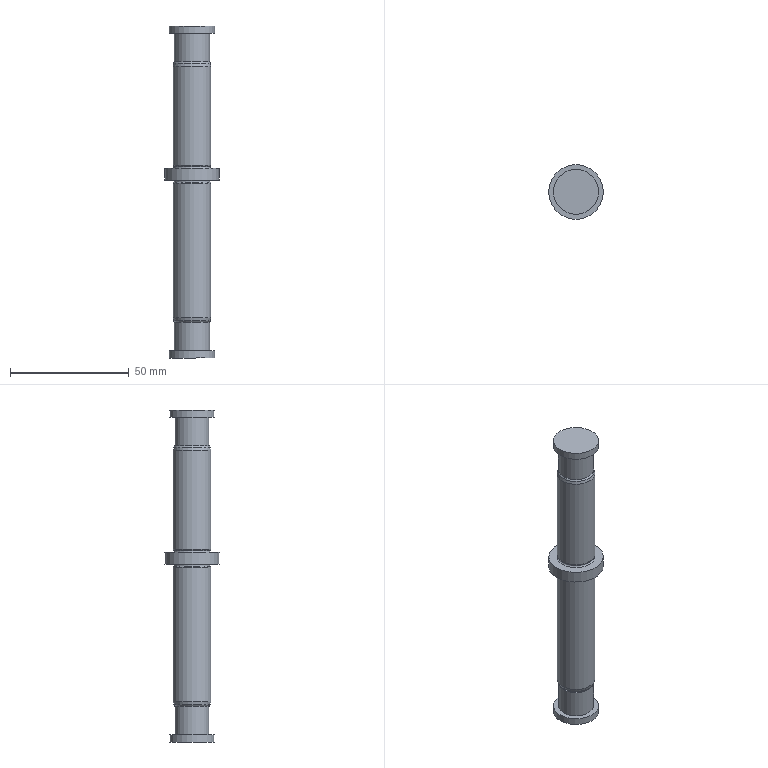Part | STEP file | 200 mesh_id1798 | 1 solid | 23 faces | box 23 x 23 x 140 mm | volume 28914 mm3 | plane 8 | cylinder 7 | torus 6 | cone 2 | commonest cylinder face diameters 14.8 x2 16 x2 19 x2 23 x1
STEP:
#1=CARTESIAN_POINT('',(-17045.208,-4095.269,118.667));
#2=VERTEX_POINT('',#1);
#3=CARTESIAN_POINT('',(-17052.884,-4095.269,118.667));
#4=DIRECTION('',(0.,0.,-1.));
#5=DIRECTION('',(1.,0.,0.));
#6=AXIS2_PLACEMENT_3D('',#3,#4,#5);
#7=CIRCLE('',#6,7.676);
#8=EDGE_CURVE('',#2,#2,#7,.T.);
#9=ORIENTED_EDGE('',*,*,#8,.T.);
#10=EDGE_LOOP('',(#9));
#11=FACE_BOUND('',#10,.T.);
#12=CARTESIAN_POINT('',(-17060.884,-4095.269,117.458));
#13=VERTEX_POINT('',#12);
#14=CARTESIAN_POINT('',(-17052.884,-4095.269,117.458));
#15=DIRECTION('',(0.,0.,-1.));
#16=DIRECTION('',(-1.,0.,0.));
#17=AXIS2_PLACEMENT_3D('',#14,#15,#16);
#18=CIRCLE('',#17,8.);
#19=EDGE_CURVE('',#13,#13,#18,.T.);
#20=ORIENTED_EDGE('',*,*,#19,.F.);
#21=EDGE_LOOP('',(#20));
#22=FACE_BOUND('',#21,.T.);
#23=CARTESIAN_POINT('',(-17052.884,-4095.269,117.458));
#24=DIRECTION('',(0.,0.,-1.));
#25=DIRECTION('',(-1.,0.,0.));
#26=AXIS2_PLACEMENT_3D('',#23,#24,#25);
#27=CONICAL_SURFACE('',#26,8.,15.);
#28=ADVANCED_FACE('',(#11,#22),#27,.T.);
#29=ORIENTED_EDGE('',*,*,#19,.T.);
#30=EDGE_LOOP('',(#29));
#31=FACE_BOUND('',#30,.T.);
#32=CARTESIAN_POINT('',(-17060.884,-4095.269,75.824));
#33=VERTEX_POINT('',#32);
#34=CARTESIAN_POINT('',(-17052.884,-4095.269,75.824));
#35=DIRECTION('',(0.,0.,-1.));
#36=DIRECTION('',(-1.,0.,0.));
#37=AXIS2_PLACEMENT_3D('',#34,#35,#36);
#38=CIRCLE('',#37,8.);
#39=EDGE_CURVE('',#33,#33,#38,.T.);
#40=ORIENTED_EDGE('',*,*,#39,.F.);
#41=EDGE_LOOP('',(#40));
#42=FACE_BOUND('',#41,.T.);
#43=CARTESIAN_POINT('',(-17052.884,-4095.269,74.458));
#44=DIRECTION('',(0.,0.,-1.));
#45=DIRECTION('',(-1.,0.,0.));
#46=AXIS2_PLACEMENT_3D('',#43,#44,#45);
#47=CYLINDRICAL_SURFACE('',#46,8.);
#48=ADVANCED_FACE('',(#31,#42),#47,.T.);
#49=ORIENTED_EDGE('',*,*,#39,.T.);
#50=EDGE_LOOP('',(#49));
#51=FACE_BOUND('',#50,.T.);
#52=CARTESIAN_POINT('',(-17060.634,-4095.269,75.391));
#53=VERTEX_POINT('',#52);
#54=CARTESIAN_POINT('',(-17052.884,-4095.269,75.391));
#55=DIRECTION('',(0.,0.,-1.));
#56=DIRECTION('',(-1.,0.,0.));
#57=AXIS2_PLACEMENT_3D('',#54,#55,#56);
#58=CIRCLE('',#57,7.75);
#59=EDGE_CURVE('',#53,#53,#58,.T.);
#60=ORIENTED_EDGE('',*,*,#59,.F.);
#61=EDGE_LOOP('',(#60));
#62=FACE_BOUND('',#61,.T.);
#63=CARTESIAN_POINT('',(-17052.884,-4095.269,75.824));
#64=DIRECTION('',(0.,0.,-1.));
#65=DIRECTION('',(-1.,0.,0.));
#66=AXIS2_PLACEMENT_3D('',#63,#64,#65);
#67=TOROIDAL_SURFACE('',#66,7.5,0.5);
#68=ADVANCED_FACE('',(#51,#62),#67,.T.);
#69=ORIENTED_EDGE('',*,*,#59,.T.);
#70=EDGE_LOOP('',(#69));
#71=FACE_BOUND('',#70,.T.);
#72=CARTESIAN_POINT('',(-17060.884,-4095.269,74.458));
#73=VERTEX_POINT('',#72);
#74=CARTESIAN_POINT('',(-17052.884,-4095.269,74.458));
#75=DIRECTION('',(0.,0.,-1.));
#76=DIRECTION('',(-1.,0.,0.));
#77=AXIS2_PLACEMENT_3D('',#74,#75,#76);
#78=CIRCLE('',#77,8.);
#79=EDGE_CURVE('',#73,#73,#78,.T.);
#80=ORIENTED_EDGE('',*,*,#79,.F.);
#81=EDGE_LOOP('',(#80));
#82=FACE_BOUND('',#81,.T.);
#83=CARTESIAN_POINT('',(-17052.884,-4095.269,74.958));
#84=DIRECTION('',(0.,0.,-1.));
#85=DIRECTION('',(-1.,0.,0.));
#86=AXIS2_PLACEMENT_3D('',#83,#84,#85);
#87=TOROIDAL_SURFACE('',#86,8.,0.5);
#88=ADVANCED_FACE('',(#71,#82),#87,.F.);
#89=ORIENTED_EDGE('',*,*,#79,.T.);
#90=EDGE_LOOP('',(#89));
#91=FACE_BOUND('',#90,.T.);
#92=CARTESIAN_POINT('',(-17064.384,-4095.269,74.458));
#93=VERTEX_POINT('',#92);
#94=CARTESIAN_POINT('',(-17052.884,-4095.269,74.458));
#95=DIRECTION('',(0.,0.,-1.));
#96=DIRECTION('',(-1.,0.,0.));
#97=AXIS2_PLACEMENT_3D('',#94,#95,#96);
#98=CIRCLE('',#97,11.5);
#99=EDGE_CURVE('',#93,#93,#98,.T.);
#100=ORIENTED_EDGE('',*,*,#99,.F.);
#101=EDGE_LOOP('',(#100));
#102=FACE_BOUND('',#101,.T.);
#103=CARTESIAN_POINT('',(-17064.384,-4095.269,74.458));
#104=DIRECTION('',(0.,0.,1.));
#105=DIRECTION('',(1.,0.,0.));
#106=AXIS2_PLACEMENT_3D('',#103,#104,#105);
#107=PLANE('',#106);
#108=ADVANCED_FACE('',(#91,#102),#107,.T.);
#109=ORIENTED_EDGE('',*,*,#99,.T.);
#110=EDGE_LOOP('',(#109));
#111=FACE_BOUND('',#110,.T.);
#112=CARTESIAN_POINT('',(-17064.384,-4095.269,69.458));
#113=VERTEX_POINT('',#112);
#114=CARTESIAN_POINT('',(-17052.884,-4095.269,69.458));
#115=DIRECTION('',(0.,0.,-1.));
#116=DIRECTION('',(-1.,0.,0.));
#117=AXIS2_PLACEMENT_3D('',#114,#115,#116);
#118=CIRCLE('',#117,11.5);
#119=EDGE_CURVE('',#113,#113,#118,.T.);
#120=ORIENTED_EDGE('',*,*,#119,.F.);
#121=EDGE_LOOP('',(#120));
#122=FACE_BOUND('',#121,.T.);
#123=CARTESIAN_POINT('',(-17052.884,-4095.269,74.458));
#124=DIRECTION('',(0.,0.,-1.));
#125=DIRECTION('',(-1.,0.,0.));
#126=AXIS2_PLACEMENT_3D('',#123,#124,#125);
#127=CYLINDRICAL_SURFACE('',#126,11.5);
#128=ADVANCED_FACE('',(#111,#122),#127,.T.);
#129=ORIENTED_EDGE('',*,*,#119,.T.);
#130=EDGE_LOOP('',(#129));
#131=FACE_BOUND('',#130,.T.);
#132=CARTESIAN_POINT('',(-17060.884,-4095.269,69.458));
#133=VERTEX_POINT('',#132);
#134=CARTESIAN_POINT('',(-17052.884,-4095.269,69.458));
#135=DIRECTION('',(0.,0.,-1.));
#136=DIRECTION('',(-1.,0.,0.));
#137=AXIS2_PLACEMENT_3D('',#134,#135,#136);
#138=CIRCLE('',#137,8.);
#139=EDGE_CURVE('',#133,#133,#138,.T.);
#140=ORIENTED_EDGE('',*,*,#139,.F.);
#141=EDGE_LOOP('',(#140));
#142=FACE_BOUND('',#141,.T.);
#143=CARTESIAN_POINT('',(-17060.884,-4095.269,69.458));
#144=DIRECTION('',(0.,0.,-1.));
#145=DIRECTION('',(-1.,0.,0.));
#146=AXIS2_PLACEMENT_3D('',#143,#144,#145);
#147=PLANE('',#146);
#148=ADVANCED_FACE('',(#131,#142),#147,.T.);
#149=ORIENTED_EDGE('',*,*,#139,.T.);
#150=EDGE_LOOP('',(#149));
#151=FACE_BOUND('',#150,.T.);
#152=CARTESIAN_POINT('',(-17060.634,-4095.269,68.525));
#153=VERTEX_POINT('',#152);
#154=CARTESIAN_POINT('',(-17052.884,-4095.269,68.525));
#155=DIRECTION('',(0.,0.,-1.));
#156=DIRECTION('',(-1.,0.,0.));
#157=AXIS2_PLACEMENT_3D('',#154,#155,#156);
#158=CIRCLE('',#157,7.75);
#159=EDGE_CURVE('',#153,#153,#158,.T.);
#160=ORIENTED_EDGE('',*,*,#159,.F.);
#161=EDGE_LOOP('',(#160));
#162=FACE_BOUND('',#161,.T.);
#163=CARTESIAN_POINT('',(-17052.884,-4095.269,68.958));
#164=DIRECTION('',(0.,0.,-1.));
#165=DIRECTION('',(-1.,0.,0.));
#166=AXIS2_PLACEMENT_3D('',#163,#164,#165);
#167=TOROIDAL_SURFACE('',#166,8.,0.5);
#168=ADVANCED_FACE('',(#151,#162),#167,.F.);
#169=ORIENTED_EDGE('',*,*,#159,.T.);
#170=EDGE_LOOP('',(#169));
#171=FACE_BOUND('',#170,.T.);
#172=CARTESIAN_POINT('',(-17060.884,-4095.269,68.092));
#173=VERTEX_POINT('',#172);
#174=CARTESIAN_POINT('',(-17052.884,-4095.269,68.092));
#175=DIRECTION('',(0.,0.,-1.));
#176=DIRECTION('',(-1.,0.,0.));
#177=AXIS2_PLACEMENT_3D('',#174,#175,#176);
#178=CIRCLE('',#177,8.);
#179=EDGE_CURVE('',#173,#173,#178,.T.);
#180=ORIENTED_EDGE('',*,*,#179,.F.);
#181=EDGE_LOOP('',(#180));
#182=FACE_BOUND('',#181,.T.);
#183=CARTESIAN_POINT('',(-17052.884,-4095.269,68.092));
#184=DIRECTION('',(0.,0.,-1.));
#185=DIRECTION('',(-1.,0.,0.));
#186=AXIS2_PLACEMENT_3D('',#183,#184,#185);
#187=TOROIDAL_SURFACE('',#186,7.5,0.5);
#188=ADVANCED_FACE('',(#171,#182),#187,.T.);
#189=ORIENTED_EDGE('',*,*,#179,.T.);
#190=EDGE_LOOP('',(#189));
#191=FACE_BOUND('',#190,.T.);
#192=CARTESIAN_POINT('',(-17060.884,-4095.269,11.458));
#193=VERTEX_POINT('',#192);
#194=CARTESIAN_POINT('',(-17052.884,-4095.269,11.458));
#195=DIRECTION('',(0.,0.,-1.));
#196=DIRECTION('',(-1.,0.,0.));
#197=AXIS2_PLACEMENT_3D('',#194,#195,#196);
#198=CIRCLE('',#197,8.);
#199=EDGE_CURVE('',#193,#193,#198,.T.);
#200=ORIENTED_EDGE('',*,*,#199,.F.);
#201=EDGE_LOOP('',(#200));
#202=FACE_BOUND('',#201,.T.);
#203=CARTESIAN_POINT('',(-17052.884,-4095.269,74.458));
#204=DIRECTION('',(0.,0.,-1.));
#205=DIRECTION('',(-1.,0.,0.));
#206=AXIS2_PLACEMENT_3D('',#203,#204,#205);
#207=CYLINDRICAL_SURFACE('',#206,8.);
#208=ADVANCED_FACE('',(#191,#202),#207,.T.);
#209=CARTESIAN_POINT('',(-17060.56,-4095.269,10.248));
#210=VERTEX_POINT('',#209);
#211=CARTESIAN_POINT('',(-17052.884,-4095.269,10.248));
#212=DIRECTION('',(0.,0.,1.));
#213=DIRECTION('',(-1.,0.,0.));
#214=AXIS2_PLACEMENT_3D('',#211,#212,#213);
#215=CIRCLE('',#214,7.676);
#216=EDGE_CURVE('',#210,#210,#215,.T.);
#217=ORIENTED_EDGE('',*,*,#216,.T.);
#218=EDGE_LOOP('',(#217));
#219=FACE_BOUND('',#218,.T.);
#220=ORIENTED_EDGE('',*,*,#199,.T.);
#221=EDGE_LOOP('',(#220));
#222=FACE_BOUND('',#221,.T.);
#223=CARTESIAN_POINT('',(-17052.884,-4095.269,9.458));
#224=DIRECTION('',(0.,0.,1.));
#225=DIRECTION('',(1.,0.,0.));
#226=AXIS2_PLACEMENT_3D('',#223,#224,#225);
#227=CONICAL_SURFACE('',#226,7.464,15.);
#228=ADVANCED_FACE('',(#219,#222),#227,.T.);
#229=CARTESIAN_POINT('',(-17046.239,-4095.269,119.458));
#230=VERTEX_POINT('',#229);
#231=CARTESIAN_POINT('',(-17052.884,-4095.269,119.458));
#232=DIRECTION('',(0.,0.,1.));
#233=DIRECTION('',(1.,0.,0.));
#234=AXIS2_PLACEMENT_3D('',#231,#232,#233);
#235=CIRCLE('',#234,6.646);
#236=EDGE_CURVE('',#230,#230,#235,.T.);
#237=ORIENTED_EDGE('',*,*,#236,.F.);
#238=EDGE_LOOP('',(#237));
#239=FACE_BOUND('',#238,.T.);
#240=ORIENTED_EDGE('',*,*,#8,.F.);
#241=EDGE_LOOP('',(#240));
#242=FACE_BOUND('',#241,.T.);
#243=CARTESIAN_POINT('',(-17052.884,-4095.269,118.391));
#244=DIRECTION('',(0.,0.,1.));
#245=DIRECTION('',(1.,0.,0.));
#246=AXIS2_PLACEMENT_3D('',#243,#244,#245);
#247=TOROIDAL_SURFACE('',#246,6.646,1.067);
#248=ADVANCED_FACE('',(#239,#242),#247,.T.);
#249=ORIENTED_EDGE('',*,*,#216,.F.);
#250=EDGE_LOOP('',(#249));
#251=FACE_BOUND('',#250,.T.);
#252=CARTESIAN_POINT('',(-17059.53,-4095.269,9.458));
#253=VERTEX_POINT('',#252);
#254=CARTESIAN_POINT('',(-17052.884,-4095.269,9.458));
#255=DIRECTION('',(0.,0.,-1.));
#256=DIRECTION('',(-1.,0.,0.));
#257=AXIS2_PLACEMENT_3D('',#254,#255,#256);
#258=CIRCLE('',#257,6.646);
#259=EDGE_CURVE('',#253,#253,#258,.T.);
#260=ORIENTED_EDGE('',*,*,#259,.F.);
#261=EDGE_LOOP('',(#260));
#262=FACE_BOUND('',#261,.T.);
#263=CARTESIAN_POINT('',(-17052.884,-4095.269,10.524));
#264=DIRECTION('',(0.,0.,-1.));
#265=DIRECTION('',(-1.,0.,0.));
#266=AXIS2_PLACEMENT_3D('',#263,#264,#265);
#267=TOROIDAL_SURFACE('',#266,6.646,1.067);
#268=ADVANCED_FACE('',(#251,#262),#267,.T.);
#269=CARTESIAN_POINT('',(-17062.384,-4095.269,134.458));
#270=VERTEX_POINT('',#269);
#271=CARTESIAN_POINT('',(-17052.884,-4095.269,134.458));
#272=DIRECTION('',(0.,0.,-1.));
#273=DIRECTION('',(-1.,0.,0.));
#274=AXIS2_PLACEMENT_3D('',#271,#272,#273);
#275=CIRCLE('',#274,9.5);
#276=EDGE_CURVE('',#270,#270,#275,.T.);
#277=ORIENTED_EDGE('',*,*,#276,.F.);
#278=EDGE_LOOP('',(#277));
#279=FACE_OUTER_BOUND('',#278,.T.);
#280=CARTESIAN_POINT('',(-17062.384,-4095.269,134.458));
#281=DIRECTION('',(0.,0.,1.));
#282=DIRECTION('',(1.,0.,0.));
#283=AXIS2_PLACEMENT_3D('',#280,#281,#282);
#284=PLANE('',#283);
#285=ADVANCED_FACE('',(#279),#284,.T.);
#286=ORIENTED_EDGE('',*,*,#276,.T.);
#287=EDGE_LOOP('',(#286));
#288=FACE_BOUND('',#287,.T.);
#289=CARTESIAN_POINT('',(-17062.384,-4095.269,131.458));
#290=VERTEX_POINT('',#289);
#291=CARTESIAN_POINT('',(-17052.884,-4095.269,131.458));
#292=DIRECTION('',(0.,0.,-1.));
#293=DIRECTION('',(-1.,0.,0.));
#294=AXIS2_PLACEMENT_3D('',#291,#292,#293);
#295=CIRCLE('',#294,9.5);
#296=EDGE_CURVE('',#290,#290,#295,.T.);
#297=ORIENTED_EDGE('',*,*,#296,.F.);
#298=EDGE_LOOP('',(#297));
#299=FACE_BOUND('',#298,.T.);
#300=CARTESIAN_POINT('',(-17052.884,-4095.269,74.458));
#301=DIRECTION('',(0.,0.,-1.));
#302=DIRECTION('',(-1.,0.,0.));
#303=AXIS2_PLACEMENT_3D('',#300,#301,#302);
#304=CYLINDRICAL_SURFACE('',#303,9.5);
#305=ADVANCED_FACE('',(#288,#299),#304,.T.);
#306=ORIENTED_EDGE('',*,*,#296,.T.);
#307=EDGE_LOOP('',(#306));
#308=FACE_BOUND('',#307,.T.);
#309=CARTESIAN_POINT('',(-17060.284,-4095.269,131.458));
#310=VERTEX_POINT('',#309);
#311=CARTESIAN_POINT('',(-17052.884,-4095.269,131.458));
#312=DIRECTION('',(0.,0.,-1.));
#313=DIRECTION('',(-1.,0.,0.));
#314=AXIS2_PLACEMENT_3D('',#311,#312,#313);
#315=CIRCLE('',#314,7.4);
#316=EDGE_CURVE('',#310,#310,#315,.T.);
#317=ORIENTED_EDGE('',*,*,#316,.F.);
#318=EDGE_LOOP('',(#317));
#319=FACE_BOUND('',#318,.T.);
#320=CARTESIAN_POINT('',(-17060.284,-4095.269,131.458));
#321=DIRECTION('',(0.,0.,-1.));
#322=DIRECTION('',(-1.,0.,0.));
#323=AXIS2_PLACEMENT_3D('',#320,#321,#322);
#324=PLANE('',#323);
#325=ADVANCED_FACE('',(#308,#319),#324,.T.);
#326=ORIENTED_EDGE('',*,*,#316,.T.);
#327=EDGE_LOOP('',(#326));
#328=FACE_BOUND('',#327,.T.);
#329=CARTESIAN_POINT('',(-17060.284,-4095.269,119.458));
#330=VERTEX_POINT('',#329);
#331=CARTESIAN_POINT('',(-17052.884,-4095.269,119.458));
#332=DIRECTION('',(0.,0.,-1.));
#333=DIRECTION('',(-1.,0.,0.));
#334=AXIS2_PLACEMENT_3D('',#331,#332,#333);
#335=CIRCLE('',#334,7.4);
#336=EDGE_CURVE('',#330,#330,#335,.T.);
#337=ORIENTED_EDGE('',*,*,#336,.F.);
#338=EDGE_LOOP('',(#337));
#339=FACE_BOUND('',#338,.T.);
#340=CARTESIAN_POINT('',(-17052.884,-4095.269,74.458));
#341=DIRECTION('',(0.,0.,-1.));
#342=DIRECTION('',(-1.,0.,0.));
#343=AXIS2_PLACEMENT_3D('',#340,#341,#342);
#344=CYLINDRICAL_SURFACE('',#343,7.4);
#345=ADVANCED_FACE('',(#328,#339),#344,.T.);
#346=ORIENTED_EDGE('',*,*,#236,.T.);
#347=EDGE_LOOP('',(#346));
#348=FACE_BOUND('',#347,.T.);
#349=ORIENTED_EDGE('',*,*,#336,.T.);
#350=EDGE_LOOP('',(#349));
#351=FACE_BOUND('',#350,.T.);
#352=CARTESIAN_POINT('',(-17052.884,-4095.269,119.458));
#353=DIRECTION('',(0.,0.,-1.));
#354=DIRECTION('',(-1.,0.,0.));
#355=AXIS2_PLACEMENT_3D('',#352,#353,#354);
#356=PLANE('',#355);
#357=ADVANCED_FACE('',(#348,#351),#356,.T.);
#358=CARTESIAN_POINT('',(-17062.384,-4095.269,-5.542));
#359=VERTEX_POINT('',#358);
#360=CARTESIAN_POINT('',(-17052.884,-4095.269,-5.542));
#361=DIRECTION('',(0.,0.,-1.));
#362=DIRECTION('',(-1.,0.,0.));
#363=AXIS2_PLACEMENT_3D('',#360,#361,#362);
#364=CIRCLE('',#363,9.5);
#365=EDGE_CURVE('',#359,#359,#364,.T.);
#366=ORIENTED_EDGE('',*,*,#365,.T.);
#367=EDGE_LOOP('',(#366));
#368=FACE_OUTER_BOUND('',#367,.T.);
#369=CARTESIAN_POINT('',(-17062.384,-4095.269,-5.542));
#370=DIRECTION('',(0.,0.,1.));
#371=DIRECTION('',(1.,0.,0.));
#372=AXIS2_PLACEMENT_3D('',#369,#370,#371);
#373=PLANE('',#372);
#374=ADVANCED_FACE('',(#368),#373,.F.);
#375=ORIENTED_EDGE('',*,*,#365,.F.);
#376=EDGE_LOOP('',(#375));
#377=FACE_BOUND('',#376,.T.);
#378=CARTESIAN_POINT('',(-17062.384,-4095.269,-2.542));
#379=VERTEX_POINT('',#378);
#380=CARTESIAN_POINT('',(-17052.884,-4095.269,-2.542));
#381=DIRECTION('',(0.,0.,-1.));
#382=DIRECTION('',(-1.,0.,0.));
#383=AXIS2_PLACEMENT_3D('',#380,#381,#382);
#384=CIRCLE('',#383,9.5);
#385=EDGE_CURVE('',#379,#379,#384,.T.);
#386=ORIENTED_EDGE('',*,*,#385,.T.);
#387=EDGE_LOOP('',(#386));
#388=FACE_BOUND('',#387,.T.);
#389=CARTESIAN_POINT('',(-17052.884,-4095.269,74.458));
#390=DIRECTION('',(0.,0.,-1.));
#391=DIRECTION('',(-1.,0.,0.));
#392=AXIS2_PLACEMENT_3D('',#389,#390,#391);
#393=CYLINDRICAL_SURFACE('',#392,9.5);
#394=ADVANCED_FACE('',(#377,#388),#393,.T.);
#395=ORIENTED_EDGE('',*,*,#385,.F.);
#396=EDGE_LOOP('',(#395));
#397=FACE_BOUND('',#396,.T.);
#398=CARTESIAN_POINT('',(-17060.284,-4095.269,-2.542));
#399=VERTEX_POINT('',#398);
#400=CARTESIAN_POINT('',(-17052.884,-4095.269,-2.542));
#401=DIRECTION('',(0.,0.,-1.));
#402=DIRECTION('',(-1.,0.,0.));
#403=AXIS2_PLACEMENT_3D('',#400,#401,#402);
#404=CIRCLE('',#403,7.4);
#405=EDGE_CURVE('',#399,#399,#404,.T.);
#406=ORIENTED_EDGE('',*,*,#405,.T.);
#407=EDGE_LOOP('',(#406));
#408=FACE_BOUND('',#407,.T.);
#409=CARTESIAN_POINT('',(-17060.284,-4095.269,-2.542));
#410=DIRECTION('',(0.,0.,-1.));
#411=DIRECTION('',(-1.,0.,0.));
#412=AXIS2_PLACEMENT_3D('',#409,#410,#411);
#413=PLANE('',#412);
#414=ADVANCED_FACE('',(#397,#408),#413,.F.);
#415=ORIENTED_EDGE('',*,*,#405,.F.);
#416=EDGE_LOOP('',(#415));
#417=FACE_BOUND('',#416,.T.);
#418=CARTESIAN_POINT('',(-17060.284,-4095.269,9.458));
#419=VERTEX_POINT('',#418);
#420=CARTESIAN_POINT('',(-17052.884,-4095.269,9.458));
#421=DIRECTION('',(0.,0.,-1.));
#422=DIRECTION('',(-1.,0.,0.));
#423=AXIS2_PLACEMENT_3D('',#420,#421,#422);
#424=CIRCLE('',#423,7.4);
#425=EDGE_CURVE('',#419,#419,#424,.T.);
#426=ORIENTED_EDGE('',*,*,#425,.T.);
#427=EDGE_LOOP('',(#426));
#428=FACE_BOUND('',#427,.T.);
#429=CARTESIAN_POINT('',(-17052.884,-4095.269,74.458));
#430=DIRECTION('',(0.,0.,-1.));
#431=DIRECTION('',(-1.,0.,0.));
#432=AXIS2_PLACEMENT_3D('',#429,#430,#431);
#433=CYLINDRICAL_SURFACE('',#432,7.4);
#434=ADVANCED_FACE('',(#417,#428),#433,.T.);
#435=ORIENTED_EDGE('',*,*,#259,.T.);
#436=EDGE_LOOP('',(#435));
#437=FACE_BOUND('',#436,.T.);
#438=ORIENTED_EDGE('',*,*,#425,.F.);
#439=EDGE_LOOP('',(#438));
#440=FACE_BOUND('',#439,.T.);
#441=CARTESIAN_POINT('',(-17052.884,-4095.269,9.458));
#442=DIRECTION('',(0.,0.,-1.));
#443=DIRECTION('',(-1.,0.,0.));
#444=AXIS2_PLACEMENT_3D('',#441,#442,#443);
#445=PLANE('',#444);
#446=ADVANCED_FACE('',(#437,#440),#445,.F.);
#447=CLOSED_SHELL('',(#28,#48,#68,#88,#108,#128,#148,#168,#188,#208,#228,#248,#268,#285,#305,#325,#345,#357,#374,#394,#414,#434,#446));
#448=MANIFOLD_SOLID_BREP('',#447);
#449=(LENGTH_UNIT()NAMED_UNIT(*)SI_UNIT(.MILLI.,.METRE.));
#450=UNCERTAINTY_MEASURE_WITH_UNIT(LENGTH_MEASURE(0.00002),#449,'','');
#451=(NAMED_UNIT(*)PLANE_ANGLE_UNIT()SI_UNIT($,.RADIAN.));
#452=PLANE_ANGLE_MEASURE_WITH_UNIT(PLANE_ANGLE_MEASURE(0.01745),#451);
#453=DIMENSIONAL_EXPONENTS(0.,0.,0.,0.,0.,0.,0.);
#454=(CONVERSION_BASED_UNIT('DEGREE',#452)NAMED_UNIT(#453)PLANE_ANGLE_UNIT());
#455=(NAMED_UNIT(*)SI_UNIT($,.STERADIAN.)SOLID_ANGLE_UNIT());
#456=(GEOMETRIC_REPRESENTATION_CONTEXT(3)GLOBAL_UNCERTAINTY_ASSIGNED_CONTEXT((#450))GLOBAL_UNIT_ASSIGNED_CONTEXT((#449,#454,#455))REPRESENTATION_CONTEXT('',''));
#457=ADVANCED_BREP_SHAPE_REPRESENTATION('',(#448),#456);